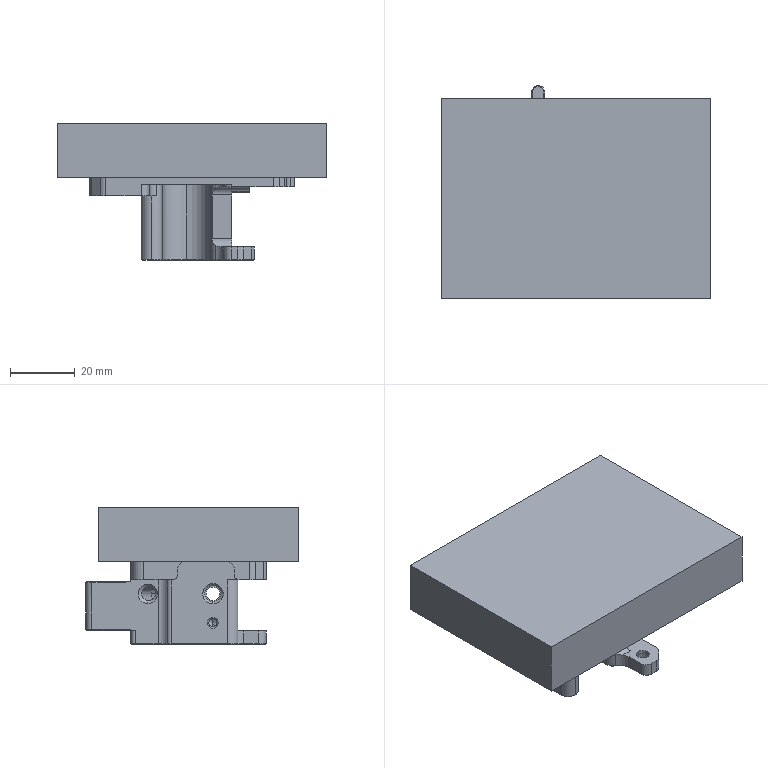CAM job | NX | 3+2 milling, drilling | part box 83.5 x 66 x 42.45 mm
Tools:
number,name,description,diameter,corner_radius,flute_length,length,flutes
1,D63,Milling Tool-5 Parameters,63.0,0.0,50.0,75.0,2
10,D10,Milling Tool-5 Parameters,10.0,0.0,50.0,75.0,2
7,D4A45,Milling Tool-5 Parameters,4.0,0.0,2.0,2.0,2
13,3.2ZT,Drilling Tool,3.2,0.0,35.0,50.0,2
12,2.5ZT,Drilling Tool,2.5,0.0,35.0,50.0,2
11,D10JING,Milling Tool-5 Parameters,10.0,0.0,50.0,75.0,2
4,D4,Milling Tool-5 Parameters,4.0,0.0,50.0,75.0,2
2,D2,Milling Tool-5 Parameters,2.0,0.0,50.0,75.0,2
15,5.0ZT,Drilling Tool,5.0,0.0,35.0,50.0,2
14,4.2ZT,Drilling Tool,4.2,0.0,35.0,50.0,2
15,D2.4XYD,Thread Mill,2.4,0.0,0.5,50.0,2
17,D4.95XYD,Thread Mill,4.95,0.0,1.0,50.0,2
15,D4.05XYD,Thread Mill,4.05,0.0,0.8,50.0,2
Operations:
program,operation,operation_type,tool,method,geometry_group,spindle_rpm,surface_speed,feed_per_tooth,feed_cut,feed_plunge,cut_length_mm,path_length_mm,cut_time_min,machine_time_min
1-68-60-35毛胚,FLOOR_WALL,VolumeBased25DMillingOperation,D63,METHOD,A,6500.0,1286.0,0.0962,1250.0,100.0,319.797,373.797,0.2558,0.2612
1-68-60-35毛胚,ADAPTIVE_MILLING,CavityMilling,D10,METHOD,A,9500.0,298.0,0.1579,3000.0,1000.0,12442.042,13050.946,4.456,4.516
1-68-60-35毛胚,ZLEVEL_PROFILE_COPY_1_COPY,ZLevelMilling,D10,METHOD,A,9500.0,298.0,0.1579,3000.0,100.0,184.276,253.576,0.0614,0.0684
1-68-60-35毛胚,ZLEVEL_PROFILE_COPY_1_COPY_COPY,ZLevelMilling,D10,METHOD,A,9500.0,298.0,0.1579,3000.0,100.0,80.945,154.345,0.027,0.0343
1-68-60-35毛胚,DRILLING_COPY_1,Operation,D4A45,METHOD,A,5000.0,94.0,0.025,250.0,0.0,51.15,360.448,0.2046,0.2355
1-68-60-35毛胚,DRILLING_COPY_COPY_1,Operation,2.5ZT,METHOD,A,2000.0,15.0,0.03,120.0,0.0,65.207,311.13,0.5434,0.568
1-68-60-35毛胚,DRILLING_COPY_COPY_1_COPY,Operation,2.5ZT,METHOD,A,2000.0,15.0,0.03,120.0,0.0,18.0,130.593,0.15,0.1613
1-68-60-35毛胚,THREAD_MILLING,ThreadMilling,D2.4XYD,METHOD,A,5000.0,37.0,0.1,1000.0,100.0,301.69,1547.11,0.3017,0.4262
1-68-60-35毛胚,THREAD_MILLING_COPY,ThreadMilling,D2.4XYD,METHOD,A,5000.0,37.0,0.1,1000.0,100.0,230.423,1017.802,0.2304,0.3092
1-68-60-35毛胚,THREAD_MILLING_COPY_COPY,ThreadMilling,D2.4XYD,METHOD,A,5000.0,37.0,0.1,1000.0,100.0,87.691,532.291,0.0877,0.1322
1-68-60-35毛胚,DRILLING_COPY_COPY_1_1,Operation,3.2ZT,METHOD,A,2000.0,15.0,0.03,120.0,0.0,34.984,208.158,0.2915,0.3089
1-68-60-35毛胚,ZLEVEL_PROFILE_COPY_COPY_1_COPY,ZLevelMilling,D10JING,METHOD,A,9500.0,298.0,0.0632,1200.0,100.0,525.406,722.112,0.4378,0.4575
1-68-60-35毛胚,ZLEVEL_PROFILE_COPY_COPY_1_COPY_COPY,ZLevelMilling,D10JING,METHOD,A,9500.0,298.0,0.0632,1200.0,100.0,22.528,94.428,0.0188,0.026
1-68-60-35毛胚,FLOOR_WALL_1_1,VolumeBased25DMillingOperation,D10JING,METHOD,A,9500.0,179.0,0.0658,1250.0,100.0,677.298,1240.209,0.5418,0.5981
1-68-60-35毛胚,FLOOR_WALL_1_1_COPY,VolumeBased25DMillingOperation,D10JING,METHOD,A,9500.0,179.0,0.0658,1250.0,100.0,84.264,156.164,0.0674,0.0746
1-68-60-35毛胚,ZLEVEL_PROFILE_COPY_1_COPY_COPY_1,ZLevelMilling,D4,METHOD,A,9500.0,119.0,0.0632,1200.0,100.0,538.991,801.769,0.4492,0.4754
1-68-60-35毛胚,ZLEVEL_PROFILE_COPY_1_COPY_COPY_1_COPY,ZLevelMilling,D4,METHOD,A,9500.0,119.0,0.0632,1200.0,100.0,270.3,527.249,0.2252,0.2509
1-68-60-35毛胚,ZLEVEL_PROFILE_COPY_1_COPY_COPY_1_COPY_COPY,ZLevelMilling,D4,METHOD,A,9500.0,119.0,0.0632,1200.0,100.0,296.898,574.882,0.2474,0.2752
1-68-60-35毛胚,ZLEVEL_PROFILE_COPY_1_COPY_1_COPY_1_1_COPY_COPY,ZLevelMilling,D4,METHOD,A,9500.0,119.0,0.0737,1400.0,800.0,131.739,285.194,0.1083,0.1237
1-68-60-35毛胚,ZLEVEL_PROFILE_COPY_1_COPY_1_COPY_1_1_COPY_COPY_COPY,ZLevelMilling,D4,METHOD,A,9500.0,119.0,0.0737,1400.0,800.0,291.609,553.054,0.2309,0.2571
1-68-60-35毛胚,ZLEVEL_PROFILE_COPY_1_COPY_COPY_1_COPY_COPY_COPY,ZLevelMilling,D2,METHOD,A,9500.0,119.0,0.0632,1200.0,100.0,427.852,584.577,0.3565,0.3722
1-68-60-35毛胚,ZLEVEL_PROFILE_1_COPY_1_COPY_COPY_1,ZLevelMilling,D4A45,METHOD,A,9500.0,179.0,0.0526,1000.0,100.0,272.53,1051.663,0.2725,0.3504
1-68-60-35毛胚,ZLEVEL_PROFILE_1_COPY_1_COPY_COPY_1_COPY,ZLevelMilling,D4A45,METHOD,A,9500.0,179.0,0.0526,1000.0,100.0,329.28,1008.028,0.3293,0.3972
1-68-60-35毛胚,ZLEVEL_PROFILE_1_COPY_1_COPY_COPY_1_COPY_COPY_1,ZLevelMilling,D4A45,METHOD,A,9500.0,179.0,0.0526,1000.0,100.0,42.821,118.721,0.0428,0.0504
1-68-60-35毛胚,ZLEVEL_PROFILE_1_COPY_1_COPY_COPY_1_COPY_COPY,ZLevelMilling,D4A45,METHOD,A,9500.0,179.0,0.0526,1000.0,100.0,89.648,271.278,0.0896,0.1078
1-68-60-35毛胚,ZLEVEL_PROFILE_1_COPY_1_COPY_COPY_1_COPY_COPY_1_COPY,ZLevelMilling,D4A45,METHOD,A,9500.0,179.0,0.0526,1000.0,100.0,35.073,122.073,0.0351,0.0438
1-68-60-35毛胚,TOOLCOMP11,VolumeBased25DMillingOperation,D10JING,METHOD,A,9500.0,179.0,0.0658,1250.0,100.0,45.694,117.594,0.0366,0.0437
1-68-60-35毛胚,TOOLCOMP15,ThreadMilling,D2.4XYD,METHOD,A,5000.0,37.0,0.085,850.0,100.0,72.976,343.396,0.0859,0.1129
1-68-60-35毛胚,TOOLCOMP15.,ThreadMilling,D2.4XYD,METHOD,A,5000.0,37.0,0.08,800.0,100.0,60.352,249.231,0.0754,0.0943
1-68-60-35毛胚,TOOLCOMP15..,ThreadMilling,D2.4XYD,METHOD,A,5000.0,37.0,0.08,800.0,100.0,21.205,95.305,0.0265,0.0339
2-68-60-35毛胚,FACE_MILLING,FaceMilling,D63,METHOD,B,6500.0,0.0,0.0,1250.0,100.0,1085.0,1321.333,0.868,0.8916
2-68-60-35毛胚,ADAPTIVE_MILLING_COPY_COPY,CavityMilling,D10,METHOD,B,9500.0,298.0,0.1579,3000.0,1000.0,18001.219,19593.314,6.01,6.169
2-68-60-35毛胚,ZLEVEL_PROFILE_COPY_COPY_1_COPY_COPY_1,ZLevelMilling,D10JING,METHOD,B,9500.0,298.0,0.0632,1200.0,100.0,189.35,281.35,0.1578,0.167
2-68-60-35毛胚,FLOOR_WALL_1_1_COPY_1,VolumeBased25DMillingOperation,D10JING,METHOD,B,9500.0,179.0,0.0658,1250.0,100.0,901.769,2651.588,0.7214,0.8964
2-68-60-35毛胚,ZLEVEL_PROFILE_COPY_1_COPY_1_COPY_1_1_COPY_COPY_COPY_1,ZLevelMilling,D4,METHOD,B,9500.0,119.0,0.0737,1400.0,800.0,1524.482,3189.184,1.225,1.391
2-68-60-35毛胚,HOLE_MILLING,CylinderMilling,D4,METHOD,B,9500.0,119.0,0.0684,1300.0,100.0,463.753,1163.621,0.3567,0.4267
2-68-60-35毛胚,HOLE_MILLING_COPY,CylinderMilling,D2,METHOD,B,9500.0,59.0,0.0526,1000.0,100.0,124.034,192.435,0.124,0.1309
2-68-60-35毛胚,ZLEVEL_PROFILE_1_COPY_1_COPY_COPY_1_COPY_COPY_1_COPY_COPY,ZLevelMilling,D4A45,METHOD,B,9500.0,179.0,0.0526,1000.0,100.0,200.843,328.591,0.2008,0.2136
2-68-60-35毛胚,ZLEVEL_PROFILE_1_COPY_1_COPY_COPY_1_COPY_COPY_1_COPY_COPY_COPY,ZLevelMilling,D4A45,METHOD,B,9500.0,179.0,0.0526,1000.0,100.0,33.634,102.934,0.0336,0.0406
2-68-60-35毛胚,ZLEVEL_PROFILE_1_COPY_1_COPY_COPY_1_COPY_COPY_1_COPY_COPY_COPY_COPY,ZLevelMilling,D4A45,METHOD,B,9500.0,179.0,0.0526,1000.0,100.0,113.51,492.474,0.1135,0.1514
2-68-60-35毛胚,ZLEVEL_PROFILE_1_COPY_1_COPY_COPY_1_COPY_COPY_1_COPY_COPY_COPY_COPY_COPY,ZLevelMilling,D4A45,METHOD,B,9500.0,179.0,0.0526,1000.0,100.0,117.18,751.087,0.1172,0.1806
2-68-60-35毛胚,ZLEVEL_PROFILE_1_COPY_1_COPY_COPY_1_COPY_COPY_1_COPY_COPY_COPY_COPY_COPY_COPY,ZLevelMilling,D4A45,METHOD,B,9500.0,179.0,0.0526,1000.0,100.0,45.937,152.937,0.0459,0.0566
3-68-60-35毛胚,DRILLING_COPY_1_COPY,Operation,D4A45,METHOD,C,5000.0,94.0,0.025,250.0,0.0,9.3,123.087,0.0372,0.0486
3-68-60-35毛胚,DRILLING_COPY_COPY_1_COPY_1,Operation,2.5ZT,METHOD,C,2000.0,15.0,0.03,120.0,0.0,9.251,110.502,0.0771,0.0872
3-68-60-35毛胚,DRILLING_COPY_COPY_1_1_COPY,Operation,5.0ZT,METHOD,C,2000.0,15.0,0.03,120.0,0.0,12.502,117.004,0.1042,0.1146
3-68-60-35毛胚,THREAD_MILLING_COPY_1,ThreadMilling,D4.95XYD,METHOD,C,3000.0,29.0,0.1667,1000.0,100.0,125.519,808.019,0.1255,0.1938
3-68-60-35毛胚,THREAD_MILLING_COPY_COPY_COPY,ThreadMilling,D2.4XYD,METHOD,C,5000.0,37.0,0.1,1000.0,100.0,84.473,660.473,0.0845,0.1421
3-68-60-35毛胚,ZLEVEL_PROFILE_COPY_1_COPY_1_COPY_1_1_COPY_COPY_COPY_1_COPY,ZLevelMilling,D4,METHOD,C,9500.0,119.0,0.0737,1400.0,800.0,1288.517,2277.836,0.9442,1.043
3-68-60-35毛胚,ZLEVEL_PROFILE_1_COPY_1_COPY_COPY_1_COPY_COPY_1_COPY_COPY_COPY_COPY_COPY_COPY_COPY,ZLevelMilling,D4A45,METHOD,C,9500.0,179.0,0.0526,1000.0,100.0,18.49,110.49,0.0185,0.0277
3-68-60-35毛胚,TOOLCOMP17,ThreadMilling,D4.95XYD,METHOD,C,3000.0,29.0,0.1333,800.0,100.0,27.56,125.06,0.0345,0.0442
3-68-60-35毛胚,TOOLCOMP15.._COPY,ThreadMilling,D2.4XYD,METHOD,C,5000.0,37.0,0.08,800.0,100.0,20.425,116.425,0.0255,0.0351
4,ADAPTIVE_MILLING_COPY,CavityMilling,D10,METHOD,D,9500.0,298.0,0.1579,3000.0,1000.0,1930.134,2475.151,0.6467,0.7012
4,DRILLING_COPY_1_COPY_COPY,Operation,D4A45,METHOD,D,5000.0,94.0,0.025,250.0,0.0,4.65,108.3,0.0186,0.029
4,DRILLING_COPY_COPY_1_1_COPY_COPY,Operation,4.2ZT,METHOD,D,2000.0,15.0,0.03,120.0,0.0,12.262,123.524,0.1022,0.1133
4,THREAD_MILLING_COPY_2_COPY,ThreadMilling,D4.05XYD,METHOD,D,3000.0,29.0,0.1667,1000.0,100.0,182.702,1123.202,0.1827,0.2768
4,ZLEVEL_PROFILE_COPY_1_COPY_1_COPY_1_1_COPY_COPY_COPY_1_COPY_1,ZLevelMilling,D4,METHOD,D,9500.0,119.0,0.0737,1400.0,800.0,193.289,492.03,0.1527,0.1826
4,FLOOR_WALL_1_1_COPY_1_COPY,VolumeBased25DMillingOperation,D4,METHOD,D,9500.0,119.0,0.0526,1000.0,100.0,413.483,1144.02,0.4135,0.4865
4,TOOLCOMP15_1,ThreadMilling,D4.05XYD,METHOD,D,3000.0,29.0,0.1333,800.0,100.0,30.493,134.993,0.0381,0.0486
5-圆回转中心对刀-20层,DRILLING,HoleDrilling,D4A45,METHOD,F,3000.0,37.0,0.025,150.0,0.0,18.0,87.851,0.06,0.067
5-圆回转中心对刀-20层,DRILLING_COPY,HoleDrilling,4.2ZT,METHOD,F,2000.0,26.0,0.025,100.0,0.0,569.524,639.375,0.3276,0.3346
5-圆回转中心对刀-20层,THREAD_MILLING_COPY_2_COPY_COPY,ThreadMilling,D4.05XYD,METHOD,F,3000.0,29.0,0.1667,1000.0,100.0,301.286,1071.966,0.3013,0.3784
5-圆回转中心对刀-20层,HOLE_MILLING_1,CylinderMilling,D4,METHOD,F,9500.0,119.0,0.0658,1250.0,100.0,347.658,435.333,0.2781,0.2869
5-圆回转中心对刀-20层,TOOLCOMP15_1_COPY,ThreadMilling,D4.05XYD,METHOD,F,3000.0,29.0,0.1333,800.0,100.0,50.298,135.929,0.0629,0.0714
6夹具,ADAPTIVE_MILLING_COPY_COPY_1,CavityMilling,D10,METHOD,E,9500.0,298.0,0.1579,3000.0,1000.0,5068.363,5130.963,1.98,1.986
6夹具,ZLEVEL_PROFILE_COPY_1_COPY_1_COPY_1_1_COPY_COPY_COPY_1_COPY_1_COPY,ZLevelMilling,D4,METHOD,E,9500.0,119.0,0.0737,1400.0,800.0,648.676,1558.81,0.5241,0.6151
6夹具,FLOOR_WALL_1_1_COPY_1_COPY_1,VolumeBased25DMillingOperation,D4,METHOD,E,9500.0,179.0,0.0658,1250.0,100.0,1379.216,1449.716,1.103,1.11
6夹具,ZLEVEL_PROFILE_1_COPY_1_COPY_COPY_1_COPY_COPY_1_COPY_COPY_COPY_COPY_COPY_COPY_COPY_COPY,ZLevelMilling,D4A45,METHOD,E,9500.0,179.0,0.0526,1000.0,100.0,199.544,259.544,0.1995,0.2055
6夹具,TOOLCOMP11_COPY,VolumeBased25DMillingOperation,D4,METHOD,E,9500.0,179.0,0.0658,1250.0,100.0,195.601,266.101,0.1565,0.1635